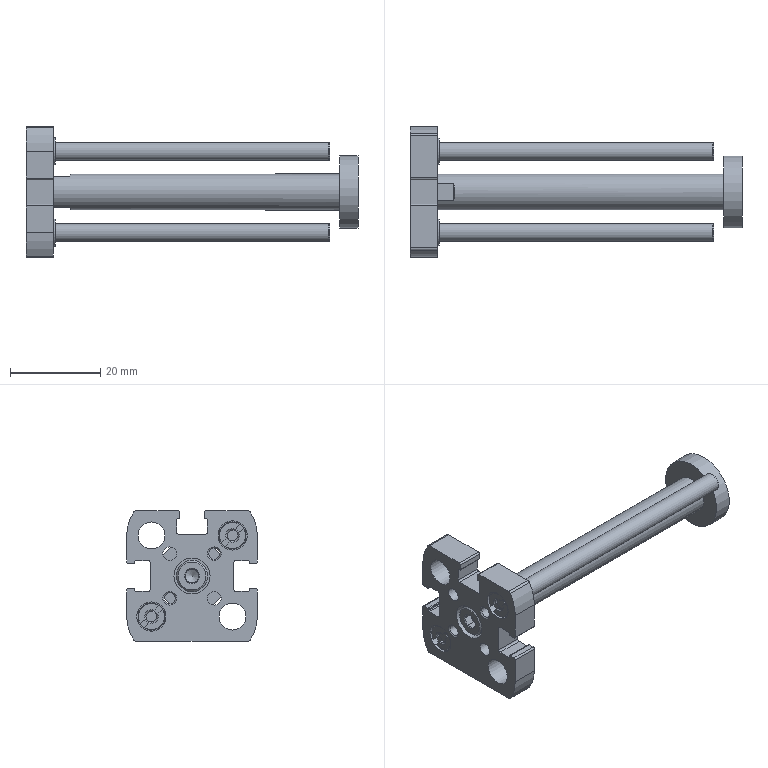Part | NX | features BREP 1 | 1 solid | 164 faces | box 73.7 x 29 x 29 mm | volume 9307 mm3 | plane 80 | cylinder 63 | cone 19 | torus 2 | commonest cylinder face diameters 0.4 x12 0.8 x12 3 x7 2.459 x6 6 x6 1.2 x4